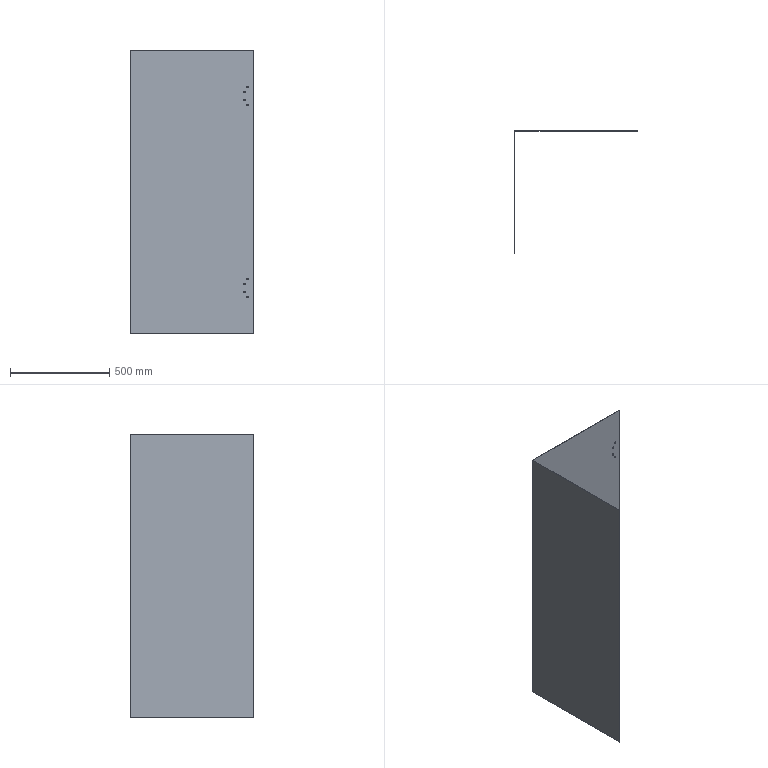Part | SolidWorks | features BaseBody 1 | 1 solid | 24 faces | box 620 x 621.122 x 1428 mm | volume 3536422 mm3 | cylinder 16 | plane 8 | commonest cylinder face diameters 8.5 x16
STEP:
#1=CARTESIAN_POINT('',(-23.395,686.977,2686.75));
#2=VERTEX_POINT('',#1);
#3=CARTESIAN_POINT('',(-23.395,686.977,2695.25));
#4=VERTEX_POINT('',#3);
#5=CARTESIAN_POINT('',(-23.395,686.977,2691.));
#6=DIRECTION('',(0.,1.,0.));
#7=DIRECTION('',(0.,0.,1.));
#8=AXIS2_PLACEMENT_3D('',#5,#6,#7);
#9=CIRCLE('',#8,4.25);
#10=EDGE_CURVE('',#2,#4,#9,.T.);
#11=ORIENTED_EDGE('',*,*,#10,.F.);
#12=CARTESIAN_POINT('',(-23.395,688.977,2686.75));
#13=VERTEX_POINT('',#12);
#14=CARTESIAN_POINT('',(-23.395,688.977,2686.75));
#15=DIRECTION('',(0.,1.,0.));
#16=VECTOR('',#15,1000.);
#17=LINE('',#14,#16);
#18=EDGE_CURVE('',#2,#13,#17,.T.);
#19=ORIENTED_EDGE('',*,*,#18,.T.);
#20=CARTESIAN_POINT('',(-23.395,688.977,2695.25));
#21=VERTEX_POINT('',#20);
#22=CARTESIAN_POINT('',(-23.395,688.977,2691.));
#23=DIRECTION('',(0.,1.,0.));
#24=DIRECTION('',(0.,0.,1.));
#25=AXIS2_PLACEMENT_3D('',#22,#23,#24);
#26=CIRCLE('',#25,4.25);
#27=EDGE_CURVE('',#13,#21,#26,.T.);
#28=ORIENTED_EDGE('',*,*,#27,.T.);
#29=CARTESIAN_POINT('',(-23.395,688.977,2695.25));
#30=DIRECTION('',(0.,1.,0.));
#31=VECTOR('',#30,1000.);
#32=LINE('',#29,#31);
#33=EDGE_CURVE('',#4,#21,#32,.T.);
#34=ORIENTED_EDGE('',*,*,#33,.F.);
#35=EDGE_LOOP('',(#11,#19,#28,#34));
#36=FACE_OUTER_BOUND('',#35,.T.);
#37=CARTESIAN_POINT('',(-23.395,688.977,2691.));
#38=DIRECTION('',(0.,1.,0.));
#39=DIRECTION('',(0.,0.,1.));
#40=AXIS2_PLACEMENT_3D('',#37,#38,#39);
#41=CYLINDRICAL_SURFACE('',#40,4.25);
#42=ADVANCED_FACE('',(#36),#41,.F.);
#43=CARTESIAN_POINT('',(-38.395,686.977,2661.75));
#44=VERTEX_POINT('',#43);
#45=CARTESIAN_POINT('',(-38.395,686.977,2670.25));
#46=VERTEX_POINT('',#45);
#47=CARTESIAN_POINT('',(-38.395,686.977,2666.));
#48=DIRECTION('',(0.,1.,0.));
#49=DIRECTION('',(0.,0.,1.));
#50=AXIS2_PLACEMENT_3D('',#47,#48,#49);
#51=CIRCLE('',#50,4.25);
#52=EDGE_CURVE('',#44,#46,#51,.T.);
#53=ORIENTED_EDGE('',*,*,#52,.F.);
#54=CARTESIAN_POINT('',(-38.395,688.977,2661.75));
#55=VERTEX_POINT('',#54);
#56=CARTESIAN_POINT('',(-38.395,688.977,2661.75));
#57=DIRECTION('',(0.,1.,0.));
#58=VECTOR('',#57,1000.);
#59=LINE('',#56,#58);
#60=EDGE_CURVE('',#44,#55,#59,.T.);
#61=ORIENTED_EDGE('',*,*,#60,.T.);
#62=CARTESIAN_POINT('',(-38.395,688.977,2670.25));
#63=VERTEX_POINT('',#62);
#64=CARTESIAN_POINT('',(-38.395,688.977,2666.));
#65=DIRECTION('',(0.,1.,0.));
#66=DIRECTION('',(0.,0.,1.));
#67=AXIS2_PLACEMENT_3D('',#64,#65,#66);
#68=CIRCLE('',#67,4.25);
#69=EDGE_CURVE('',#55,#63,#68,.T.);
#70=ORIENTED_EDGE('',*,*,#69,.T.);
#71=CARTESIAN_POINT('',(-38.395,688.977,2670.25));
#72=DIRECTION('',(0.,1.,0.));
#73=VECTOR('',#72,1000.);
#74=LINE('',#71,#73);
#75=EDGE_CURVE('',#46,#63,#74,.T.);
#76=ORIENTED_EDGE('',*,*,#75,.F.);
#77=EDGE_LOOP('',(#53,#61,#70,#76));
#78=FACE_OUTER_BOUND('',#77,.T.);
#79=CARTESIAN_POINT('',(-38.395,688.977,2666.));
#80=DIRECTION('',(0.,1.,0.));
#81=DIRECTION('',(0.,0.,1.));
#82=AXIS2_PLACEMENT_3D('',#79,#80,#81);
#83=CYLINDRICAL_SURFACE('',#82,4.25);
#84=ADVANCED_FACE('',(#78),#83,.F.);
#85=CARTESIAN_POINT('',(-38.395,686.977,2621.75));
#86=VERTEX_POINT('',#85);
#87=CARTESIAN_POINT('',(-38.395,686.977,2630.25));
#88=VERTEX_POINT('',#87);
#89=CARTESIAN_POINT('',(-38.395,686.977,2626.));
#90=DIRECTION('',(0.,1.,0.));
#91=DIRECTION('',(0.,0.,1.));
#92=AXIS2_PLACEMENT_3D('',#89,#90,#91);
#93=CIRCLE('',#92,4.25);
#94=EDGE_CURVE('',#86,#88,#93,.T.);
#95=ORIENTED_EDGE('',*,*,#94,.F.);
#96=CARTESIAN_POINT('',(-38.395,688.977,2621.75));
#97=VERTEX_POINT('',#96);
#98=CARTESIAN_POINT('',(-38.395,688.977,2621.75));
#99=DIRECTION('',(0.,1.,0.));
#100=VECTOR('',#99,1000.);
#101=LINE('',#98,#100);
#102=EDGE_CURVE('',#86,#97,#101,.T.);
#103=ORIENTED_EDGE('',*,*,#102,.T.);
#104=CARTESIAN_POINT('',(-38.395,688.977,2630.25));
#105=VERTEX_POINT('',#104);
#106=CARTESIAN_POINT('',(-38.395,688.977,2626.));
#107=DIRECTION('',(0.,1.,0.));
#108=DIRECTION('',(0.,0.,1.));
#109=AXIS2_PLACEMENT_3D('',#106,#107,#108);
#110=CIRCLE('',#109,4.25);
#111=EDGE_CURVE('',#97,#105,#110,.T.);
#112=ORIENTED_EDGE('',*,*,#111,.T.);
#113=CARTESIAN_POINT('',(-38.395,688.977,2630.25));
#114=DIRECTION('',(0.,1.,0.));
#115=VECTOR('',#114,1000.);
#116=LINE('',#113,#115);
#117=EDGE_CURVE('',#88,#105,#116,.T.);
#118=ORIENTED_EDGE('',*,*,#117,.F.);
#119=EDGE_LOOP('',(#95,#103,#112,#118));
#120=FACE_OUTER_BOUND('',#119,.T.);
#121=CARTESIAN_POINT('',(-38.395,688.977,2626.));
#122=DIRECTION('',(0.,1.,0.));
#123=DIRECTION('',(0.,0.,1.));
#124=AXIS2_PLACEMENT_3D('',#121,#122,#123);
#125=CYLINDRICAL_SURFACE('',#124,4.25);
#126=ADVANCED_FACE('',(#120),#125,.F.);
#127=CARTESIAN_POINT('',(-23.395,686.977,2596.75));
#128=VERTEX_POINT('',#127);
#129=CARTESIAN_POINT('',(-23.395,686.977,2605.25));
#130=VERTEX_POINT('',#129);
#131=CARTESIAN_POINT('',(-23.395,686.977,2601.));
#132=DIRECTION('',(0.,1.,0.));
#133=DIRECTION('',(0.,0.,1.));
#134=AXIS2_PLACEMENT_3D('',#131,#132,#133);
#135=CIRCLE('',#134,4.25);
#136=EDGE_CURVE('',#128,#130,#135,.T.);
#137=ORIENTED_EDGE('',*,*,#136,.F.);
#138=CARTESIAN_POINT('',(-23.395,688.977,2596.75));
#139=VERTEX_POINT('',#138);
#140=CARTESIAN_POINT('',(-23.395,688.977,2596.75));
#141=DIRECTION('',(0.,1.,0.));
#142=VECTOR('',#141,1000.);
#143=LINE('',#140,#142);
#144=EDGE_CURVE('',#128,#139,#143,.T.);
#145=ORIENTED_EDGE('',*,*,#144,.T.);
#146=CARTESIAN_POINT('',(-23.395,688.977,2605.25));
#147=VERTEX_POINT('',#146);
#148=CARTESIAN_POINT('',(-23.395,688.977,2601.));
#149=DIRECTION('',(0.,1.,0.));
#150=DIRECTION('',(0.,0.,1.));
#151=AXIS2_PLACEMENT_3D('',#148,#149,#150);
#152=CIRCLE('',#151,4.25);
#153=EDGE_CURVE('',#139,#147,#152,.T.);
#154=ORIENTED_EDGE('',*,*,#153,.T.);
#155=CARTESIAN_POINT('',(-23.395,688.977,2605.25));
#156=DIRECTION('',(0.,1.,0.));
#157=VECTOR('',#156,1000.);
#158=LINE('',#155,#157);
#159=EDGE_CURVE('',#130,#147,#158,.T.);
#160=ORIENTED_EDGE('',*,*,#159,.F.);
#161=EDGE_LOOP('',(#137,#145,#154,#160));
#162=FACE_OUTER_BOUND('',#161,.T.);
#163=CARTESIAN_POINT('',(-23.395,688.977,2601.));
#164=DIRECTION('',(0.,1.,0.));
#165=DIRECTION('',(0.,0.,1.));
#166=AXIS2_PLACEMENT_3D('',#163,#164,#165);
#167=CYLINDRICAL_SURFACE('',#166,4.25);
#168=ADVANCED_FACE('',(#162),#167,.F.);
#169=CARTESIAN_POINT('',(-23.395,686.977,1718.75));
#170=VERTEX_POINT('',#169);
#171=CARTESIAN_POINT('',(-23.395,686.977,1727.25));
#172=VERTEX_POINT('',#171);
#173=CARTESIAN_POINT('',(-23.395,686.977,1723.));
#174=DIRECTION('',(0.,1.,0.));
#175=DIRECTION('',(0.,0.,1.));
#176=AXIS2_PLACEMENT_3D('',#173,#174,#175);
#177=CIRCLE('',#176,4.25);
#178=EDGE_CURVE('',#170,#172,#177,.T.);
#179=ORIENTED_EDGE('',*,*,#178,.F.);
#180=CARTESIAN_POINT('',(-23.395,688.977,1718.75));
#181=VERTEX_POINT('',#180);
#182=CARTESIAN_POINT('',(-23.395,688.977,1718.75));
#183=DIRECTION('',(0.,1.,0.));
#184=VECTOR('',#183,1000.);
#185=LINE('',#182,#184);
#186=EDGE_CURVE('',#170,#181,#185,.T.);
#187=ORIENTED_EDGE('',*,*,#186,.T.);
#188=CARTESIAN_POINT('',(-23.395,688.977,1727.25));
#189=VERTEX_POINT('',#188);
#190=CARTESIAN_POINT('',(-23.395,688.977,1723.));
#191=DIRECTION('',(0.,1.,0.));
#192=DIRECTION('',(0.,0.,1.));
#193=AXIS2_PLACEMENT_3D('',#190,#191,#192);
#194=CIRCLE('',#193,4.25);
#195=EDGE_CURVE('',#181,#189,#194,.T.);
#196=ORIENTED_EDGE('',*,*,#195,.T.);
#197=CARTESIAN_POINT('',(-23.395,688.977,1727.25));
#198=DIRECTION('',(0.,1.,0.));
#199=VECTOR('',#198,1000.);
#200=LINE('',#197,#199);
#201=EDGE_CURVE('',#172,#189,#200,.T.);
#202=ORIENTED_EDGE('',*,*,#201,.F.);
#203=EDGE_LOOP('',(#179,#187,#196,#202));
#204=FACE_OUTER_BOUND('',#203,.T.);
#205=CARTESIAN_POINT('',(-23.395,688.977,1723.));
#206=DIRECTION('',(0.,1.,0.));
#207=DIRECTION('',(0.,0.,1.));
#208=AXIS2_PLACEMENT_3D('',#205,#206,#207);
#209=CYLINDRICAL_SURFACE('',#208,4.25);
#210=ADVANCED_FACE('',(#204),#209,.F.);
#211=CARTESIAN_POINT('',(-38.395,686.977,1693.75));
#212=VERTEX_POINT('',#211);
#213=CARTESIAN_POINT('',(-38.395,686.977,1702.25));
#214=VERTEX_POINT('',#213);
#215=CARTESIAN_POINT('',(-38.395,686.977,1698.));
#216=DIRECTION('',(0.,1.,0.));
#217=DIRECTION('',(0.,0.,1.));
#218=AXIS2_PLACEMENT_3D('',#215,#216,#217);
#219=CIRCLE('',#218,4.25);
#220=EDGE_CURVE('',#212,#214,#219,.T.);
#221=ORIENTED_EDGE('',*,*,#220,.F.);
#222=CARTESIAN_POINT('',(-38.395,688.977,1693.75));
#223=VERTEX_POINT('',#222);
#224=CARTESIAN_POINT('',(-38.395,688.977,1693.75));
#225=DIRECTION('',(0.,1.,0.));
#226=VECTOR('',#225,1000.);
#227=LINE('',#224,#226);
#228=EDGE_CURVE('',#212,#223,#227,.T.);
#229=ORIENTED_EDGE('',*,*,#228,.T.);
#230=CARTESIAN_POINT('',(-38.395,688.977,1702.25));
#231=VERTEX_POINT('',#230);
#232=CARTESIAN_POINT('',(-38.395,688.977,1698.));
#233=DIRECTION('',(0.,1.,0.));
#234=DIRECTION('',(0.,0.,1.));
#235=AXIS2_PLACEMENT_3D('',#232,#233,#234);
#236=CIRCLE('',#235,4.25);
#237=EDGE_CURVE('',#223,#231,#236,.T.);
#238=ORIENTED_EDGE('',*,*,#237,.T.);
#239=CARTESIAN_POINT('',(-38.395,688.977,1702.25));
#240=DIRECTION('',(0.,1.,0.));
#241=VECTOR('',#240,1000.);
#242=LINE('',#239,#241);
#243=EDGE_CURVE('',#214,#231,#242,.T.);
#244=ORIENTED_EDGE('',*,*,#243,.F.);
#245=EDGE_LOOP('',(#221,#229,#238,#244));
#246=FACE_OUTER_BOUND('',#245,.T.);
#247=CARTESIAN_POINT('',(-38.395,688.977,1698.));
#248=DIRECTION('',(0.,1.,0.));
#249=DIRECTION('',(0.,0.,1.));
#250=AXIS2_PLACEMENT_3D('',#247,#248,#249);
#251=CYLINDRICAL_SURFACE('',#250,4.25);
#252=ADVANCED_FACE('',(#246),#251,.F.);
#253=CARTESIAN_POINT('',(-38.395,686.977,1653.75));
#254=VERTEX_POINT('',#253);
#255=CARTESIAN_POINT('',(-38.395,686.977,1662.25));
#256=VERTEX_POINT('',#255);
#257=CARTESIAN_POINT('',(-38.395,686.977,1658.));
#258=DIRECTION('',(0.,1.,0.));
#259=DIRECTION('',(0.,0.,1.));
#260=AXIS2_PLACEMENT_3D('',#257,#258,#259);
#261=CIRCLE('',#260,4.25);
#262=EDGE_CURVE('',#254,#256,#261,.T.);
#263=ORIENTED_EDGE('',*,*,#262,.F.);
#264=CARTESIAN_POINT('',(-38.395,688.977,1653.75));
#265=VERTEX_POINT('',#264);
#266=CARTESIAN_POINT('',(-38.395,688.977,1653.75));
#267=DIRECTION('',(0.,1.,0.));
#268=VECTOR('',#267,1000.);
#269=LINE('',#266,#268);
#270=EDGE_CURVE('',#254,#265,#269,.T.);
#271=ORIENTED_EDGE('',*,*,#270,.T.);
#272=CARTESIAN_POINT('',(-38.395,688.977,1662.25));
#273=VERTEX_POINT('',#272);
#274=CARTESIAN_POINT('',(-38.395,688.977,1658.));
#275=DIRECTION('',(0.,1.,0.));
#276=DIRECTION('',(0.,0.,1.));
#277=AXIS2_PLACEMENT_3D('',#274,#275,#276);
#278=CIRCLE('',#277,4.25);
#279=EDGE_CURVE('',#265,#273,#278,.T.);
#280=ORIENTED_EDGE('',*,*,#279,.T.);
#281=CARTESIAN_POINT('',(-38.395,688.977,1662.25));
#282=DIRECTION('',(0.,1.,0.));
#283=VECTOR('',#282,1000.);
#284=LINE('',#281,#283);
#285=EDGE_CURVE('',#256,#273,#284,.T.);
#286=ORIENTED_EDGE('',*,*,#285,.F.);
#287=EDGE_LOOP('',(#263,#271,#280,#286));
#288=FACE_OUTER_BOUND('',#287,.T.);
#289=CARTESIAN_POINT('',(-38.395,688.977,1658.));
#290=DIRECTION('',(0.,1.,0.));
#291=DIRECTION('',(0.,0.,1.));
#292=AXIS2_PLACEMENT_3D('',#289,#290,#291);
#293=CYLINDRICAL_SURFACE('',#292,4.25);
#294=ADVANCED_FACE('',(#288),#293,.F.);
#295=CARTESIAN_POINT('',(-23.395,686.977,1628.75));
#296=VERTEX_POINT('',#295);
#297=CARTESIAN_POINT('',(-23.395,686.977,1637.25));
#298=VERTEX_POINT('',#297);
#299=CARTESIAN_POINT('',(-23.395,686.977,1633.));
#300=DIRECTION('',(0.,1.,0.));
#301=DIRECTION('',(0.,0.,1.));
#302=AXIS2_PLACEMENT_3D('',#299,#300,#301);
#303=CIRCLE('',#302,4.25);
#304=EDGE_CURVE('',#296,#298,#303,.T.);
#305=ORIENTED_EDGE('',*,*,#304,.F.);
#306=CARTESIAN_POINT('',(-23.395,688.977,1628.75));
#307=VERTEX_POINT('',#306);
#308=CARTESIAN_POINT('',(-23.395,688.977,1628.75));
#309=DIRECTION('',(0.,1.,0.));
#310=VECTOR('',#309,1000.);
#311=LINE('',#308,#310);
#312=EDGE_CURVE('',#296,#307,#311,.T.);
#313=ORIENTED_EDGE('',*,*,#312,.T.);
#314=CARTESIAN_POINT('',(-23.395,688.977,1637.25));
#315=VERTEX_POINT('',#314);
#316=CARTESIAN_POINT('',(-23.395,688.977,1633.));
#317=DIRECTION('',(0.,1.,0.));
#318=DIRECTION('',(0.,0.,1.));
#319=AXIS2_PLACEMENT_3D('',#316,#317,#318);
#320=CIRCLE('',#319,4.25);
#321=EDGE_CURVE('',#307,#315,#320,.T.);
#322=ORIENTED_EDGE('',*,*,#321,.T.);
#323=CARTESIAN_POINT('',(-23.395,688.977,1637.25));
#324=DIRECTION('',(0.,1.,0.));
#325=VECTOR('',#324,1000.);
#326=LINE('',#323,#325);
#327=EDGE_CURVE('',#298,#315,#326,.T.);
#328=ORIENTED_EDGE('',*,*,#327,.F.);
#329=EDGE_LOOP('',(#305,#313,#322,#328));
#330=FACE_OUTER_BOUND('',#329,.T.);
#331=CARTESIAN_POINT('',(-23.395,688.977,1633.));
#332=DIRECTION('',(0.,1.,0.));
#333=DIRECTION('',(0.,0.,1.));
#334=AXIS2_PLACEMENT_3D('',#331,#332,#333);
#335=CYLINDRICAL_SURFACE('',#334,4.25);
#336=ADVANCED_FACE('',(#330),#335,.F.);
#337=CARTESIAN_POINT('',(-23.395,686.977,2691.));
#338=DIRECTION('',(0.,1.,0.));
#339=DIRECTION('',(0.,0.,1.));
#340=AXIS2_PLACEMENT_3D('',#337,#338,#339);
#341=CIRCLE('',#340,4.25);
#342=EDGE_CURVE('',#4,#2,#341,.T.);
#343=ORIENTED_EDGE('',*,*,#342,.T.);
#344=ORIENTED_EDGE('',*,*,#10,.T.);
#345=EDGE_LOOP('',(#343,#344));
#346=FACE_BOUND('',#345,.T.);
#347=CARTESIAN_POINT('',(-38.395,686.977,2666.));
#348=DIRECTION('',(0.,1.,0.));
#349=DIRECTION('',(0.,0.,1.));
#350=AXIS2_PLACEMENT_3D('',#347,#348,#349);
#351=CIRCLE('',#350,4.25);
#352=EDGE_CURVE('',#46,#44,#351,.T.);
#353=ORIENTED_EDGE('',*,*,#352,.T.);
#354=ORIENTED_EDGE('',*,*,#52,.T.);
#355=EDGE_LOOP('',(#353,#354));
#356=FACE_BOUND('',#355,.T.);
#357=CARTESIAN_POINT('',(-38.395,686.977,2626.));
#358=DIRECTION('',(0.,1.,0.));
#359=DIRECTION('',(0.,0.,1.));
#360=AXIS2_PLACEMENT_3D('',#357,#358,#359);
#361=CIRCLE('',#360,4.25);
#362=EDGE_CURVE('',#88,#86,#361,.T.);
#363=ORIENTED_EDGE('',*,*,#362,.T.);
#364=ORIENTED_EDGE('',*,*,#94,.T.);
#365=EDGE_LOOP('',(#363,#364));
#366=FACE_BOUND('',#365,.T.);
#367=CARTESIAN_POINT('',(-23.395,686.977,2601.));
#368=DIRECTION('',(0.,1.,0.));
#369=DIRECTION('',(0.,0.,1.));
#370=AXIS2_PLACEMENT_3D('',#367,#368,#369);
#371=CIRCLE('',#370,4.25);
#372=EDGE_CURVE('',#130,#128,#371,.T.);
#373=ORIENTED_EDGE('',*,*,#372,.T.);
#374=ORIENTED_EDGE('',*,*,#136,.T.);
#375=EDGE_LOOP('',(#373,#374));
#376=FACE_BOUND('',#375,.T.);
#377=CARTESIAN_POINT('',(-23.395,686.977,1723.));
#378=DIRECTION('',(0.,1.,0.));
#379=DIRECTION('',(0.,0.,1.));
#380=AXIS2_PLACEMENT_3D('',#377,#378,#379);
#381=CIRCLE('',#380,4.25);
#382=EDGE_CURVE('',#172,#170,#381,.T.);
#383=ORIENTED_EDGE('',*,*,#382,.T.);
#384=ORIENTED_EDGE('',*,*,#178,.T.);
#385=EDGE_LOOP('',(#383,#384));
#386=FACE_BOUND('',#385,.T.);
#387=CARTESIAN_POINT('',(-38.395,686.977,1698.));
#388=DIRECTION('',(0.,1.,0.));
#389=DIRECTION('',(0.,0.,1.));
#390=AXIS2_PLACEMENT_3D('',#387,#388,#389);
#391=CIRCLE('',#390,4.25);
#392=EDGE_CURVE('',#214,#212,#391,.T.);
#393=ORIENTED_EDGE('',*,*,#392,.T.);
#394=ORIENTED_EDGE('',*,*,#220,.T.);
#395=EDGE_LOOP('',(#393,#394));
#396=FACE_BOUND('',#395,.T.);
#397=CARTESIAN_POINT('',(-38.395,686.977,1658.));
#398=DIRECTION('',(0.,1.,0.));
#399=DIRECTION('',(0.,0.,1.));
#400=AXIS2_PLACEMENT_3D('',#397,#398,#399);
#401=CIRCLE('',#400,4.25);
#402=EDGE_CURVE('',#256,#254,#401,.T.);
#403=ORIENTED_EDGE('',*,*,#402,.T.);
#404=ORIENTED_EDGE('',*,*,#262,.T.);
#405=EDGE_LOOP('',(#403,#404));
#406=FACE_BOUND('',#405,.T.);
#407=CARTESIAN_POINT('',(-23.395,686.977,1633.));
#408=DIRECTION('',(0.,1.,0.));
#409=DIRECTION('',(0.,0.,1.));
#410=AXIS2_PLACEMENT_3D('',#407,#408,#409);
#411=CIRCLE('',#410,4.25);
#412=EDGE_CURVE('',#298,#296,#411,.T.);
#413=ORIENTED_EDGE('',*,*,#412,.T.);
#414=ORIENTED_EDGE('',*,*,#304,.T.);
#415=EDGE_LOOP('',(#413,#414));
#416=FACE_BOUND('',#415,.T.);
#417=CARTESIAN_POINT('',(6.605,686.977,2876.));
#418=VERTEX_POINT('',#417);
#419=CARTESIAN_POINT('',(6.605,686.977,1448.));
#420=VERTEX_POINT('',#419);
#421=CARTESIAN_POINT('',(6.605,686.977,2876.));
#422=DIRECTION('',(0.,0.,-1.));
#423=VECTOR('',#422,1000.);
#424=LINE('',#421,#423);
#425=EDGE_CURVE('',#418,#420,#424,.T.);
#426=ORIENTED_EDGE('',*,*,#425,.F.);
#427=CARTESIAN_POINT('',(-611.395,686.977,2876.));
#428=VERTEX_POINT('',#427);
#429=CARTESIAN_POINT('',(0.,686.977,2876.));
#430=DIRECTION('',(1.,0.,0.));
#431=VECTOR('',#430,1000.);
#432=LINE('',#429,#431);
#433=EDGE_CURVE('',#428,#418,#432,.T.);
#434=ORIENTED_EDGE('',*,*,#433,.F.);
#435=CARTESIAN_POINT('',(-611.395,686.977,1448.));
#436=VERTEX_POINT('',#435);
#437=CARTESIAN_POINT('',(-611.395,686.977,2876.));
#438=DIRECTION('',(0.,0.,-1.));
#439=VECTOR('',#438,1000.);
#440=LINE('',#437,#439);
#441=EDGE_CURVE('',#428,#436,#440,.T.);
#442=ORIENTED_EDGE('',*,*,#441,.T.);
#443=CARTESIAN_POINT('',(550.605,686.977,1448.));
#444=DIRECTION('',(1.,0.,0.));
#445=VECTOR('',#444,1000.);
#446=LINE('',#443,#445);
#447=EDGE_CURVE('',#436,#420,#446,.T.);
#448=ORIENTED_EDGE('',*,*,#447,.T.);
#449=EDGE_LOOP('',(#426,#434,#442,#448));
#450=FACE_OUTER_BOUND('',#449,.T.);
#451=CARTESIAN_POINT('',(550.605,686.977,2876.));
#452=DIRECTION('',(0.,1.,0.));
#453=DIRECTION('',(0.,0.,1.));
#454=AXIS2_PLACEMENT_3D('',#451,#452,#453);
#455=PLANE('',#454);
#456=ADVANCED_FACE('',(#346,#356,#366,#376,#386,#396,#406,#416,#450),#455,.F.);
#457=CARTESIAN_POINT('',(-23.395,688.977,2691.));
#458=DIRECTION('',(0.,1.,0.));
#459=DIRECTION('',(0.,0.,1.));
#460=AXIS2_PLACEMENT_3D('',#457,#458,#459);
#461=CIRCLE('',#460,4.25);
#462=EDGE_CURVE('',#21,#13,#461,.T.);
#463=ORIENTED_EDGE('',*,*,#462,.F.);
#464=ORIENTED_EDGE('',*,*,#27,.F.);
#465=EDGE_LOOP('',(#463,#464));
#466=FACE_BOUND('',#465,.T.);
#467=CARTESIAN_POINT('',(-38.395,688.977,2666.));
#468=DIRECTION('',(0.,1.,0.));
#469=DIRECTION('',(0.,0.,1.));
#470=AXIS2_PLACEMENT_3D('',#467,#468,#469);
#471=CIRCLE('',#470,4.25);
#472=EDGE_CURVE('',#63,#55,#471,.T.);
#473=ORIENTED_EDGE('',*,*,#472,.F.);
#474=ORIENTED_EDGE('',*,*,#69,.F.);
#475=EDGE_LOOP('',(#473,#474));
#476=FACE_BOUND('',#475,.T.);
#477=CARTESIAN_POINT('',(-38.395,688.977,2626.));
#478=DIRECTION('',(0.,1.,0.));
#479=DIRECTION('',(0.,0.,1.));
#480=AXIS2_PLACEMENT_3D('',#477,#478,#479);
#481=CIRCLE('',#480,4.25);
#482=EDGE_CURVE('',#105,#97,#481,.T.);
#483=ORIENTED_EDGE('',*,*,#482,.F.);
#484=ORIENTED_EDGE('',*,*,#111,.F.);
#485=EDGE_LOOP('',(#483,#484));
#486=FACE_BOUND('',#485,.T.);
#487=CARTESIAN_POINT('',(-23.395,688.977,2601.));
#488=DIRECTION('',(0.,1.,0.));
#489=DIRECTION('',(0.,0.,1.));
#490=AXIS2_PLACEMENT_3D('',#487,#488,#489);
#491=CIRCLE('',#490,4.25);
#492=EDGE_CURVE('',#147,#139,#491,.T.);
#493=ORIENTED_EDGE('',*,*,#492,.F.);
#494=ORIENTED_EDGE('',*,*,#153,.F.);
#495=EDGE_LOOP('',(#493,#494));
#496=FACE_BOUND('',#495,.T.);
#497=CARTESIAN_POINT('',(-23.395,688.977,1723.));
#498=DIRECTION('',(0.,1.,0.));
#499=DIRECTION('',(0.,0.,1.));
#500=AXIS2_PLACEMENT_3D('',#497,#498,#499);
#501=CIRCLE('',#500,4.25);
#502=EDGE_CURVE('',#189,#181,#501,.T.);
#503=ORIENTED_EDGE('',*,*,#502,.F.);
#504=ORIENTED_EDGE('',*,*,#195,.F.);
#505=EDGE_LOOP('',(#503,#504));
#506=FACE_BOUND('',#505,.T.);
#507=CARTESIAN_POINT('',(-38.395,688.977,1698.));
#508=DIRECTION('',(0.,1.,0.));
#509=DIRECTION('',(0.,0.,1.));
#510=AXIS2_PLACEMENT_3D('',#507,#508,#509);
#511=CIRCLE('',#510,4.25);
#512=EDGE_CURVE('',#231,#223,#511,.T.);
#513=ORIENTED_EDGE('',*,*,#512,.F.);
#514=ORIENTED_EDGE('',*,*,#237,.F.);
#515=EDGE_LOOP('',(#513,#514));
#516=FACE_BOUND('',#515,.T.);
#517=CARTESIAN_POINT('',(-38.395,688.977,1658.));
#518=DIRECTION('',(0.,1.,0.));
#519=DIRECTION('',(0.,0.,1.));
#520=AXIS2_PLACEMENT_3D('',#517,#518,#519);
#521=CIRCLE('',#520,4.25);
#522=EDGE_CURVE('',#273,#265,#521,.T.);
#523=ORIENTED_EDGE('',*,*,#522,.F.);
#524=ORIENTED_EDGE('',*,*,#279,.F.);
#525=EDGE_LOOP('',(#523,#524));
#526=FACE_BOUND('',#525,.T.);
#527=CARTESIAN_POINT('',(-23.395,688.977,1633.));
#528=DIRECTION('',(0.,1.,0.));
#529=DIRECTION('',(0.,0.,1.));
#530=AXIS2_PLACEMENT_3D('',#527,#528,#529);
#531=CIRCLE('',#530,4.25);
#532=EDGE_CURVE('',#315,#307,#531,.T.);
#533=ORIENTED_EDGE('',*,*,#532,.F.);
#534=ORIENTED_EDGE('',*,*,#321,.F.);
#535=EDGE_LOOP('',(#533,#534));
#536=FACE_BOUND('',#535,.T.);
#537=CARTESIAN_POINT('',(-613.395,688.977,1448.));
#538=VERTEX_POINT('',#537);
#539=CARTESIAN_POINT('',(6.605,688.977,1448.));
#540=VERTEX_POINT('',#539);
#541=CARTESIAN_POINT('',(550.605,688.977,1448.));
#542=DIRECTION('',(1.,0.,0.));
#543=VECTOR('',#542,1000.);
#544=LINE('',#541,#543);
#545=EDGE_CURVE('',#538,#540,#544,.T.);
#546=ORIENTED_EDGE('',*,*,#545,.F.);
#547=CARTESIAN_POINT('',(-613.395,688.977,2876.));
#548=VERTEX_POINT('',#547);
#549=CARTESIAN_POINT('',(-613.395,688.977,2876.));
#550=DIRECTION('',(0.,0.,-1.));
#551=VECTOR('',#550,1000.);
#552=LINE('',#549,#551);
#553=EDGE_CURVE('',#548,#538,#552,.T.);
#554=ORIENTED_EDGE('',*,*,#553,.F.);
#555=CARTESIAN_POINT('',(6.605,688.977,2876.));
#556=VERTEX_POINT('',#555);
#557=CARTESIAN_POINT('',(0.,688.977,2876.));
#558=DIRECTION('',(1.,0.,0.));
#559=VECTOR('',#558,1000.);
#560=LINE('',#557,#559);
#561=EDGE_CURVE('',#548,#556,#560,.T.);
#562=ORIENTED_EDGE('',*,*,#561,.T.);
#563=CARTESIAN_POINT('',(6.605,688.977,2876.));
#564=DIRECTION('',(0.,0.,-1.));
#565=VECTOR('',#564,1000.);
#566=LINE('',#563,#565);
#567=EDGE_CURVE('',#556,#540,#566,.T.);
#568=ORIENTED_EDGE('',*,*,#567,.T.);
#569=EDGE_LOOP('',(#546,#554,#562,#568));
#570=FACE_OUTER_BOUND('',#569,.T.);
#571=CARTESIAN_POINT('',(550.605,688.977,2876.));
#572=DIRECTION('',(0.,1.,0.));
#573=DIRECTION('',(0.,0.,1.));
#574=AXIS2_PLACEMENT_3D('',#571,#572,#573);
#575=PLANE('',#574);
#576=ADVANCED_FACE('',(#466,#476,#486,#496,#506,#516,#526,#536,#570),#575,.T.);
#577=CARTESIAN_POINT('',(6.605,0.,2876.));
#578=DIRECTION('',(0.,-1.,0.));
#579=VECTOR('',#578,1000.);
#580=LINE('',#577,#579);
#581=EDGE_CURVE('',#556,#418,#580,.T.);
#582=ORIENTED_EDGE('',*,*,#581,.F.);
#583=ORIENTED_EDGE('',*,*,#561,.F.);
#584=CARTESIAN_POINT('',(-613.395,68.977,2876.));
#585=VERTEX_POINT('',#584);
#586=CARTESIAN_POINT('',(-613.395,658.977,2876.));
#587=DIRECTION('',(0.,1.,0.));
#588=VECTOR('',#587,1000.);
#589=LINE('',#586,#588);
#590=EDGE_CURVE('',#585,#548,#589,.T.);
#591=ORIENTED_EDGE('',*,*,#590,.F.);
#592=CARTESIAN_POINT('',(-611.395,68.977,2876.));
#593=VERTEX_POINT('',#592);
#594=CARTESIAN_POINT('',(0.,68.977,2876.));
#595=DIRECTION('',(-1.,0.,0.));
#596=VECTOR('',#595,1000.);
#597=LINE('',#594,#596);
#598=EDGE_CURVE('',#593,#585,#597,.T.);
#599=ORIENTED_EDGE('',*,*,#598,.F.);
#600=CARTESIAN_POINT('',(-611.395,0.,2876.));
#601=DIRECTION('',(0.,1.,0.));
#602=VECTOR('',#601,1000.);
#603=LINE('',#600,#602);
#604=EDGE_CURVE('',#593,#428,#603,.T.);
#605=ORIENTED_EDGE('',*,*,#604,.T.);
#606=ORIENTED_EDGE('',*,*,#433,.T.);
#607=EDGE_LOOP('',(#582,#583,#591,#599,#605,#606));
#608=FACE_OUTER_BOUND('',#607,.T.);
#609=CARTESIAN_POINT('',(0.,0.,2876.));
#610=DIRECTION('',(0.,0.,-1.));
#611=DIRECTION('',(-1.,0.,0.));
#612=AXIS2_PLACEMENT_3D('',#609,#610,#611);
#613=PLANE('',#612);
#614=ADVANCED_FACE('',(#608),#613,.F.);
#615=ORIENTED_EDGE('',*,*,#447,.F.);
#616=CARTESIAN_POINT('',(-611.395,67.856,1448.));
#617=VERTEX_POINT('',#616);
#618=CARTESIAN_POINT('',(-611.395,658.977,1448.));
#619=DIRECTION('',(0.,1.,0.));
#620=VECTOR('',#619,1000.);
#621=LINE('',#618,#620);
#622=EDGE_CURVE('',#617,#436,#621,.T.);
#623=ORIENTED_EDGE('',*,*,#622,.F.);
#624=CARTESIAN_POINT('',(-613.395,67.856,1448.));
#625=VERTEX_POINT('',#624);
#626=CARTESIAN_POINT('',(-611.395,67.856,1448.));
#627=DIRECTION('',(1.,0.,0.));
#628=VECTOR('',#627,1000.);
#629=LINE('',#626,#628);
#630=EDGE_CURVE('',#625,#617,#629,.T.);
#631=ORIENTED_EDGE('',*,*,#630,.F.);
#632=CARTESIAN_POINT('',(-613.395,658.977,1448.));
#633=DIRECTION('',(0.,1.,0.));
#634=VECTOR('',#633,1000.);
#635=LINE('',#632,#634);
#636=EDGE_CURVE('',#625,#538,#635,.T.);
#637=ORIENTED_EDGE('',*,*,#636,.T.);
#638=ORIENTED_EDGE('',*,*,#545,.T.);
#639=CARTESIAN_POINT('',(6.605,556.977,1448.));
#640=DIRECTION('',(0.,1.,0.));
#641=VECTOR('',#640,1000.);
#642=LINE('',#639,#641);
#643=EDGE_CURVE('',#420,#540,#642,.T.);
#644=ORIENTED_EDGE('',*,*,#643,.F.);
#645=EDGE_LOOP('',(#615,#623,#631,#637,#638,#644));
#646=FACE_OUTER_BOUND('',#645,.T.);
#647=CARTESIAN_POINT('',(-611.395,556.977,1448.));
#648=DIRECTION('',(0.,0.,1.));
#649=DIRECTION('',(1.,0.,0.));
#650=AXIS2_PLACEMENT_3D('',#647,#648,#649);
#651=PLANE('',#650);
#652=ADVANCED_FACE('',(#646),#651,.F.);
#653=ORIENTED_EDGE('',*,*,#553,.T.);
#654=ORIENTED_EDGE('',*,*,#636,.F.);
#655=CARTESIAN_POINT('',(-613.395,68.978,2876.463));
#656=DIRECTION('',(0.,0.0007854,1.));
#657=VECTOR('',#656,1000.);
#658=LINE('',#655,#657);
#659=EDGE_CURVE('',#625,#585,#658,.T.);
#660=ORIENTED_EDGE('',*,*,#659,.T.);
#661=ORIENTED_EDGE('',*,*,#590,.T.);
#662=EDGE_LOOP('',(#653,#654,#660,#661));
#663=FACE_OUTER_BOUND('',#662,.T.);
#664=CARTESIAN_POINT('',(-613.395,658.977,2876.));
#665=DIRECTION('',(-1.,0.,0.));
#666=DIRECTION('',(0.,-1.,0.));
#667=AXIS2_PLACEMENT_3D('',#664,#665,#666);
#668=PLANE('',#667);
#669=ADVANCED_FACE('',(#663),#668,.T.);
#670=ORIENTED_EDGE('',*,*,#622,.T.);
#671=ORIENTED_EDGE('',*,*,#441,.F.);
#672=ORIENTED_EDGE('',*,*,#604,.F.);
#673=CARTESIAN_POINT('',(-611.395,68.978,2876.463));
#674=DIRECTION('',(0.,0.0007854,1.));
#675=VECTOR('',#674,1000.);
#676=LINE('',#673,#675);
#677=EDGE_CURVE('',#617,#593,#676,.T.);
#678=ORIENTED_EDGE('',*,*,#677,.F.);
#679=EDGE_LOOP('',(#670,#671,#672,#678));
#680=FACE_OUTER_BOUND('',#679,.T.);
#681=CARTESIAN_POINT('',(-611.395,658.977,2876.));
#682=DIRECTION('',(-1.,0.,0.));
#683=DIRECTION('',(0.,-1.,0.));
#684=AXIS2_PLACEMENT_3D('',#681,#682,#683);
#685=PLANE('',#684);
#686=ADVANCED_FACE('',(#680),#685,.F.);
#687=ORIENTED_EDGE('',*,*,#630,.T.);
#688=ORIENTED_EDGE('',*,*,#677,.T.);
#689=ORIENTED_EDGE('',*,*,#598,.T.);
#690=ORIENTED_EDGE('',*,*,#659,.F.);
#691=EDGE_LOOP('',(#687,#688,#689,#690));
#692=FACE_OUTER_BOUND('',#691,.T.);
#693=CARTESIAN_POINT('',(550.615,67.856,1448.));
#694=DIRECTION('',(0.,-1.,0.0007854));
#695=DIRECTION('',(0.,-0.0007854,-1.));
#696=AXIS2_PLACEMENT_3D('',#693,#694,#695);
#697=PLANE('',#696);
#698=ADVANCED_FACE('',(#692),#697,.T.);
#699=ORIENTED_EDGE('',*,*,#567,.F.);
#700=ORIENTED_EDGE('',*,*,#581,.T.);
#701=ORIENTED_EDGE('',*,*,#425,.T.);
#702=ORIENTED_EDGE('',*,*,#643,.T.);
#703=EDGE_LOOP('',(#699,#700,#701,#702));
#704=FACE_OUTER_BOUND('',#703,.T.);
#705=CARTESIAN_POINT('',(6.605,-551.033,2950.727));
#706=DIRECTION('',(1.,0.,0.));
#707=DIRECTION('',(0.,0.,-1.));
#708=AXIS2_PLACEMENT_3D('',#705,#706,#707);
#709=PLANE('',#708);
#710=ADVANCED_FACE('',(#704),#709,.T.);
#711=ORIENTED_EDGE('',*,*,#312,.F.);
#712=ORIENTED_EDGE('',*,*,#412,.F.);
#713=ORIENTED_EDGE('',*,*,#327,.T.);
#714=ORIENTED_EDGE('',*,*,#532,.T.);
#715=EDGE_LOOP('',(#711,#712,#713,#714));
#716=FACE_OUTER_BOUND('',#715,.T.);
#717=CARTESIAN_POINT('',(-23.395,688.977,1633.));
#718=DIRECTION('',(0.,1.,0.));
#719=DIRECTION('',(0.,0.,1.));
#720=AXIS2_PLACEMENT_3D('',#717,#718,#719);
#721=CYLINDRICAL_SURFACE('',#720,4.25);
#722=ADVANCED_FACE('',(#716),#721,.F.);
#723=ORIENTED_EDGE('',*,*,#270,.F.);
#724=ORIENTED_EDGE('',*,*,#402,.F.);
#725=ORIENTED_EDGE('',*,*,#285,.T.);
#726=ORIENTED_EDGE('',*,*,#522,.T.);
#727=EDGE_LOOP('',(#723,#724,#725,#726));
#728=FACE_OUTER_BOUND('',#727,.T.);
#729=CARTESIAN_POINT('',(-38.395,688.977,1658.));
#730=DIRECTION('',(0.,1.,0.));
#731=DIRECTION('',(0.,0.,1.));
#732=AXIS2_PLACEMENT_3D('',#729,#730,#731);
#733=CYLINDRICAL_SURFACE('',#732,4.25);
#734=ADVANCED_FACE('',(#728),#733,.F.);
#735=ORIENTED_EDGE('',*,*,#228,.F.);
#736=ORIENTED_EDGE('',*,*,#392,.F.);
#737=ORIENTED_EDGE('',*,*,#243,.T.);
#738=ORIENTED_EDGE('',*,*,#512,.T.);
#739=EDGE_LOOP('',(#735,#736,#737,#738));
#740=FACE_OUTER_BOUND('',#739,.T.);
#741=CARTESIAN_POINT('',(-38.395,688.977,1698.));
#742=DIRECTION('',(0.,1.,0.));
#743=DIRECTION('',(0.,0.,1.));
#744=AXIS2_PLACEMENT_3D('',#741,#742,#743);
#745=CYLINDRICAL_SURFACE('',#744,4.25);
#746=ADVANCED_FACE('',(#740),#745,.F.);
#747=ORIENTED_EDGE('',*,*,#186,.F.);
#748=ORIENTED_EDGE('',*,*,#382,.F.);
#749=ORIENTED_EDGE('',*,*,#201,.T.);
#750=ORIENTED_EDGE('',*,*,#502,.T.);
#751=EDGE_LOOP('',(#747,#748,#749,#750));
#752=FACE_OUTER_BOUND('',#751,.T.);
#753=CARTESIAN_POINT('',(-23.395,688.977,1723.));
#754=DIRECTION('',(0.,1.,0.));
#755=DIRECTION('',(0.,0.,1.));
#756=AXIS2_PLACEMENT_3D('',#753,#754,#755);
#757=CYLINDRICAL_SURFACE('',#756,4.25);
#758=ADVANCED_FACE('',(#752),#757,.F.);
#759=ORIENTED_EDGE('',*,*,#144,.F.);
#760=ORIENTED_EDGE('',*,*,#372,.F.);
#761=ORIENTED_EDGE('',*,*,#159,.T.);
#762=ORIENTED_EDGE('',*,*,#492,.T.);
#763=EDGE_LOOP('',(#759,#760,#761,#762));
#764=FACE_OUTER_BOUND('',#763,.T.);
#765=CARTESIAN_POINT('',(-23.395,688.977,2601.));
#766=DIRECTION('',(0.,1.,0.));
#767=DIRECTION('',(0.,0.,1.));
#768=AXIS2_PLACEMENT_3D('',#765,#766,#767);
#769=CYLINDRICAL_SURFACE('',#768,4.25);
#770=ADVANCED_FACE('',(#764),#769,.F.);
#771=ORIENTED_EDGE('',*,*,#102,.F.);
#772=ORIENTED_EDGE('',*,*,#362,.F.);
#773=ORIENTED_EDGE('',*,*,#117,.T.);
#774=ORIENTED_EDGE('',*,*,#482,.T.);
#775=EDGE_LOOP('',(#771,#772,#773,#774));
#776=FACE_OUTER_BOUND('',#775,.T.);
#777=CARTESIAN_POINT('',(-38.395,688.977,2626.));
#778=DIRECTION('',(0.,1.,0.));
#779=DIRECTION('',(0.,0.,1.));
#780=AXIS2_PLACEMENT_3D('',#777,#778,#779);
#781=CYLINDRICAL_SURFACE('',#780,4.25);
#782=ADVANCED_FACE('',(#776),#781,.F.);
#783=ORIENTED_EDGE('',*,*,#60,.F.);
#784=ORIENTED_EDGE('',*,*,#352,.F.);
#785=ORIENTED_EDGE('',*,*,#75,.T.);
#786=ORIENTED_EDGE('',*,*,#472,.T.);
#787=EDGE_LOOP('',(#783,#784,#785,#786));
#788=FACE_OUTER_BOUND('',#787,.T.);
#789=CARTESIAN_POINT('',(-38.395,688.977,2666.));
#790=DIRECTION('',(0.,1.,0.));
#791=DIRECTION('',(0.,0.,1.));
#792=AXIS2_PLACEMENT_3D('',#789,#790,#791);
#793=CYLINDRICAL_SURFACE('',#792,4.25);
#794=ADVANCED_FACE('',(#788),#793,.F.);
#795=ORIENTED_EDGE('',*,*,#18,.F.);
#796=ORIENTED_EDGE('',*,*,#342,.F.);
#797=ORIENTED_EDGE('',*,*,#33,.T.);
#798=ORIENTED_EDGE('',*,*,#462,.T.);
#799=EDGE_LOOP('',(#795,#796,#797,#798));
#800=FACE_OUTER_BOUND('',#799,.T.);
#801=CARTESIAN_POINT('',(-23.395,688.977,2691.));
#802=DIRECTION('',(0.,1.,0.));
#803=DIRECTION('',(0.,0.,1.));
#804=AXIS2_PLACEMENT_3D('',#801,#802,#803);
#805=CYLINDRICAL_SURFACE('',#804,4.25);
#806=ADVANCED_FACE('',(#800),#805,.F.);
#807=CLOSED_SHELL('',(#42,#84,#126,#168,#210,#252,#294,#336,#456,#576,#614,#652,#669,#686,#698,#710,#722,#734,#746,#758,#770,#782,#794,#806));
#808=MANIFOLD_SOLID_BREP('',#807);
#809=CARTESIAN_POINT('',(0.,0.,0.));
#810=DIRECTION('',(0.,0.,1.));
#811=DIRECTION('',(1.,0.,0.));
#812=AXIS2_PLACEMENT_3D('',#809,#810,#811);
#813=(LENGTH_UNIT()NAMED_UNIT(*)SI_UNIT(.MILLI.,.METRE.));
#814=UNCERTAINTY_MEASURE_WITH_UNIT(LENGTH_MEASURE(0.00001),#813,'','');
#815=(NAMED_UNIT(*)PLANE_ANGLE_UNIT()SI_UNIT($,.RADIAN.));
#816=(NAMED_UNIT(*)SI_UNIT($,.STERADIAN.)SOLID_ANGLE_UNIT());
#817=(GEOMETRIC_REPRESENTATION_CONTEXT(3)GLOBAL_UNCERTAINTY_ASSIGNED_CONTEXT((#814))GLOBAL_UNIT_ASSIGNED_CONTEXT((#813,#815,#816))REPRESENTATION_CONTEXT('',''));
#818=ADVANCED_BREP_SHAPE_REPRESENTATION('',(#808,#812),#817);